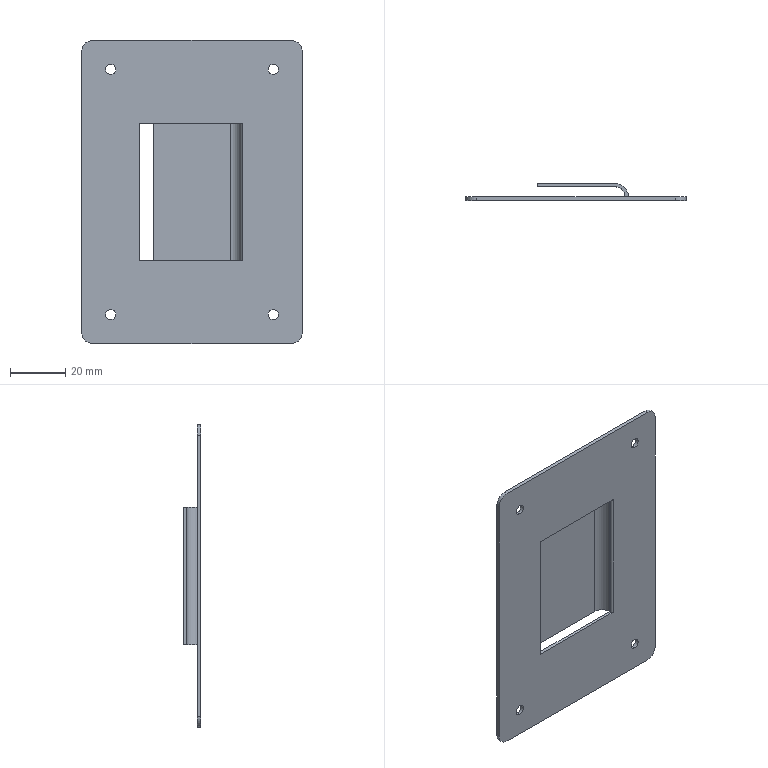Part | SolidWorks | features FlatPattern 1, ICE 1, SMBaseFlange 1, SheetMetal 1 | 1 solid | 30 faces | box 80 x 6.2 x 110 mm | volume 10376 mm3 | cylinder 15 | plane 15 | commonest cylinder face diameters 3.664 x8 8 x4 1.2 x1 7.6 x1 10 x1
STEP:
#1=CARTESIAN_POINT('',(-29.5,-1.2,-46.332));
#2=VERTEX_POINT('',#1);
#3=CARTESIAN_POINT('',(-29.5,-1.2,-42.668));
#4=VERTEX_POINT('',#3);
#5=CARTESIAN_POINT('',(-29.5,-1.2,-44.5));
#6=DIRECTION('',(0.,1.,0.));
#7=DIRECTION('',(0.,0.,-1.));
#8=AXIS2_PLACEMENT_3D('',#5,#6,#7);
#9=CIRCLE('',#8,1.832);
#10=EDGE_CURVE('',#2,#4,#9,.T.);
#11=ORIENTED_EDGE('',*,*,#10,.F.);
#12=CARTESIAN_POINT('',(-29.5,0.,-46.332));
#13=VERTEX_POINT('',#12);
#14=CARTESIAN_POINT('',(-29.5,-1.2,-46.332));
#15=DIRECTION('',(0.,1.,0.));
#16=VECTOR('',#15,1000.);
#17=LINE('',#14,#16);
#18=EDGE_CURVE('',#2,#13,#17,.T.);
#19=ORIENTED_EDGE('',*,*,#18,.T.);
#20=CARTESIAN_POINT('',(-29.5,0.,-42.668));
#21=VERTEX_POINT('',#20);
#22=CARTESIAN_POINT('',(-29.5,0.,-44.5));
#23=DIRECTION('',(0.,1.,0.));
#24=DIRECTION('',(0.,0.,-1.));
#25=AXIS2_PLACEMENT_3D('',#22,#23,#24);
#26=CIRCLE('',#25,1.832);
#27=EDGE_CURVE('',#13,#21,#26,.T.);
#28=ORIENTED_EDGE('',*,*,#27,.T.);
#29=CARTESIAN_POINT('',(-29.5,-1.2,-42.668));
#30=DIRECTION('',(0.,1.,0.));
#31=VECTOR('',#30,1000.);
#32=LINE('',#29,#31);
#33=EDGE_CURVE('',#4,#21,#32,.T.);
#34=ORIENTED_EDGE('',*,*,#33,.F.);
#35=EDGE_LOOP('',(#11,#19,#28,#34));
#36=FACE_OUTER_BOUND('',#35,.T.);
#37=CARTESIAN_POINT('',(-29.5,-1.2,-44.5));
#38=DIRECTION('',(0.,1.,0.));
#39=DIRECTION('',(0.,0.,1.));
#40=AXIS2_PLACEMENT_3D('',#37,#38,#39);
#41=CYLINDRICAL_SURFACE('',#40,1.832);
#42=ADVANCED_FACE('',(#36),#41,.F.);
#43=CARTESIAN_POINT('',(29.5,-1.2,-46.332));
#44=VERTEX_POINT('',#43);
#45=CARTESIAN_POINT('',(29.5,-1.2,-42.668));
#46=VERTEX_POINT('',#45);
#47=CARTESIAN_POINT('',(29.5,-1.2,-44.5));
#48=DIRECTION('',(0.,1.,0.));
#49=DIRECTION('',(0.,0.,1.));
#50=AXIS2_PLACEMENT_3D('',#47,#48,#49);
#51=CIRCLE('',#50,1.832);
#52=EDGE_CURVE('',#44,#46,#51,.T.);
#53=ORIENTED_EDGE('',*,*,#52,.F.);
#54=CARTESIAN_POINT('',(29.5,0.,-46.332));
#55=VERTEX_POINT('',#54);
#56=CARTESIAN_POINT('',(29.5,-1.2,-46.332));
#57=DIRECTION('',(0.,1.,0.));
#58=VECTOR('',#57,1000.);
#59=LINE('',#56,#58);
#60=EDGE_CURVE('',#44,#55,#59,.T.);
#61=ORIENTED_EDGE('',*,*,#60,.T.);
#62=CARTESIAN_POINT('',(29.5,0.,-42.668));
#63=VERTEX_POINT('',#62);
#64=CARTESIAN_POINT('',(29.5,0.,-44.5));
#65=DIRECTION('',(0.,1.,0.));
#66=DIRECTION('',(0.,0.,1.));
#67=AXIS2_PLACEMENT_3D('',#64,#65,#66);
#68=CIRCLE('',#67,1.832);
#69=EDGE_CURVE('',#55,#63,#68,.T.);
#70=ORIENTED_EDGE('',*,*,#69,.T.);
#71=CARTESIAN_POINT('',(29.5,-1.2,-42.668));
#72=DIRECTION('',(0.,1.,0.));
#73=VECTOR('',#72,1000.);
#74=LINE('',#71,#73);
#75=EDGE_CURVE('',#46,#63,#74,.T.);
#76=ORIENTED_EDGE('',*,*,#75,.F.);
#77=EDGE_LOOP('',(#53,#61,#70,#76));
#78=FACE_OUTER_BOUND('',#77,.T.);
#79=CARTESIAN_POINT('',(29.5,-1.2,-44.5));
#80=DIRECTION('',(0.,1.,0.));
#81=DIRECTION('',(0.,0.,1.));
#82=AXIS2_PLACEMENT_3D('',#79,#80,#81);
#83=CYLINDRICAL_SURFACE('',#82,1.832);
#84=ADVANCED_FACE('',(#78),#83,.F.);
#85=CARTESIAN_POINT('',(29.5,-1.2,42.668));
#86=VERTEX_POINT('',#85);
#87=CARTESIAN_POINT('',(29.5,-1.2,46.332));
#88=VERTEX_POINT('',#87);
#89=CARTESIAN_POINT('',(29.5,-1.2,44.5));
#90=DIRECTION('',(0.,1.,0.));
#91=DIRECTION('',(0.,0.,-1.));
#92=AXIS2_PLACEMENT_3D('',#89,#90,#91);
#93=CIRCLE('',#92,1.832);
#94=EDGE_CURVE('',#86,#88,#93,.T.);
#95=ORIENTED_EDGE('',*,*,#94,.F.);
#96=CARTESIAN_POINT('',(29.5,0.,42.668));
#97=VERTEX_POINT('',#96);
#98=CARTESIAN_POINT('',(29.5,-1.2,42.668));
#99=DIRECTION('',(0.,1.,0.));
#100=VECTOR('',#99,1000.);
#101=LINE('',#98,#100);
#102=EDGE_CURVE('',#86,#97,#101,.T.);
#103=ORIENTED_EDGE('',*,*,#102,.T.);
#104=CARTESIAN_POINT('',(29.5,0.,46.332));
#105=VERTEX_POINT('',#104);
#106=CARTESIAN_POINT('',(29.5,0.,44.5));
#107=DIRECTION('',(0.,1.,0.));
#108=DIRECTION('',(0.,0.,-1.));
#109=AXIS2_PLACEMENT_3D('',#106,#107,#108);
#110=CIRCLE('',#109,1.832);
#111=EDGE_CURVE('',#97,#105,#110,.T.);
#112=ORIENTED_EDGE('',*,*,#111,.T.);
#113=CARTESIAN_POINT('',(29.5,-1.2,46.332));
#114=DIRECTION('',(0.,1.,0.));
#115=VECTOR('',#114,1000.);
#116=LINE('',#113,#115);
#117=EDGE_CURVE('',#88,#105,#116,.T.);
#118=ORIENTED_EDGE('',*,*,#117,.F.);
#119=EDGE_LOOP('',(#95,#103,#112,#118));
#120=FACE_OUTER_BOUND('',#119,.T.);
#121=CARTESIAN_POINT('',(29.5,-1.2,44.5));
#122=DIRECTION('',(0.,1.,0.));
#123=DIRECTION('',(0.,0.,1.));
#124=AXIS2_PLACEMENT_3D('',#121,#122,#123);
#125=CYLINDRICAL_SURFACE('',#124,1.832);
#126=ADVANCED_FACE('',(#120),#125,.F.);
#127=CARTESIAN_POINT('',(-29.5,-1.2,42.668));
#128=VERTEX_POINT('',#127);
#129=CARTESIAN_POINT('',(-29.5,-1.2,46.332));
#130=VERTEX_POINT('',#129);
#131=CARTESIAN_POINT('',(-29.5,-1.2,44.5));
#132=DIRECTION('',(0.,1.,0.));
#133=DIRECTION('',(0.,0.,1.));
#134=AXIS2_PLACEMENT_3D('',#131,#132,#133);
#135=CIRCLE('',#134,1.832);
#136=EDGE_CURVE('',#128,#130,#135,.T.);
#137=ORIENTED_EDGE('',*,*,#136,.F.);
#138=CARTESIAN_POINT('',(-29.5,0.,42.668));
#139=VERTEX_POINT('',#138);
#140=CARTESIAN_POINT('',(-29.5,-1.2,42.668));
#141=DIRECTION('',(0.,1.,0.));
#142=VECTOR('',#141,1000.);
#143=LINE('',#140,#142);
#144=EDGE_CURVE('',#128,#139,#143,.T.);
#145=ORIENTED_EDGE('',*,*,#144,.T.);
#146=CARTESIAN_POINT('',(-29.5,0.,46.332));
#147=VERTEX_POINT('',#146);
#148=CARTESIAN_POINT('',(-29.5,0.,44.5));
#149=DIRECTION('',(0.,1.,0.));
#150=DIRECTION('',(0.,0.,1.));
#151=AXIS2_PLACEMENT_3D('',#148,#149,#150);
#152=CIRCLE('',#151,1.832);
#153=EDGE_CURVE('',#139,#147,#152,.T.);
#154=ORIENTED_EDGE('',*,*,#153,.T.);
#155=CARTESIAN_POINT('',(-29.5,-1.2,46.332));
#156=DIRECTION('',(0.,1.,0.));
#157=VECTOR('',#156,1000.);
#158=LINE('',#155,#157);
#159=EDGE_CURVE('',#130,#147,#158,.T.);
#160=ORIENTED_EDGE('',*,*,#159,.F.);
#161=EDGE_LOOP('',(#137,#145,#154,#160));
#162=FACE_OUTER_BOUND('',#161,.T.);
#163=CARTESIAN_POINT('',(-29.5,-1.2,44.5));
#164=DIRECTION('',(0.,1.,0.));
#165=DIRECTION('',(0.,0.,1.));
#166=AXIS2_PLACEMENT_3D('',#163,#164,#165);
#167=CYLINDRICAL_SURFACE('',#166,1.832);
#168=ADVANCED_FACE('',(#162),#167,.F.);
#169=CARTESIAN_POINT('',(17.8,0.,25.));
#170=VERTEX_POINT('',#169);
#171=CARTESIAN_POINT('',(17.8,-0.6,25.));
#172=VERTEX_POINT('',#171);
#173=CARTESIAN_POINT('',(17.8,-0.6,25.));
#174=DIRECTION('',(0.,-1.,0.));
#175=VECTOR('',#174,1000.);
#176=LINE('',#173,#175);
#177=EDGE_CURVE('',#170,#172,#176,.T.);
#178=ORIENTED_EDGE('',*,*,#177,.T.);
#179=CARTESIAN_POINT('',(18.4,-1.2,25.));
#180=VERTEX_POINT('',#179);
#181=CARTESIAN_POINT('',(18.4,-0.6,25.));
#182=DIRECTION('',(0.,0.,1.));
#183=DIRECTION('',(1.,0.,0.));
#184=AXIS2_PLACEMENT_3D('',#181,#182,#183);
#185=CIRCLE('',#184,0.6);
#186=EDGE_CURVE('',#172,#180,#185,.T.);
#187=ORIENTED_EDGE('',*,*,#186,.T.);
#188=CARTESIAN_POINT('',(-19.,-1.2,25.));
#189=VERTEX_POINT('',#188);
#190=CARTESIAN_POINT('',(-19.,-1.2,25.));
#191=DIRECTION('',(1.,0.,0.));
#192=VECTOR('',#191,1000.);
#193=LINE('',#190,#192);
#194=EDGE_CURVE('',#189,#180,#193,.T.);
#195=ORIENTED_EDGE('',*,*,#194,.F.);
#196=CARTESIAN_POINT('',(-19.,0.,25.));
#197=VERTEX_POINT('',#196);
#198=CARTESIAN_POINT('',(-19.,-1.2,25.));
#199=DIRECTION('',(0.,1.,0.));
#200=VECTOR('',#199,1000.);
#201=LINE('',#198,#200);
#202=EDGE_CURVE('',#189,#197,#201,.T.);
#203=ORIENTED_EDGE('',*,*,#202,.T.);
#204=CARTESIAN_POINT('',(-19.,0.,25.));
#205=DIRECTION('',(1.,0.,0.));
#206=VECTOR('',#205,1000.);
#207=LINE('',#204,#206);
#208=EDGE_CURVE('',#197,#170,#207,.T.);
#209=ORIENTED_EDGE('',*,*,#208,.T.);
#210=EDGE_LOOP('',(#178,#187,#195,#203,#209));
#211=FACE_OUTER_BOUND('',#210,.T.);
#212=CARTESIAN_POINT('',(-19.,-1.2,25.));
#213=DIRECTION('',(0.,0.,1.));
#214=DIRECTION('',(1.,0.,0.));
#215=AXIS2_PLACEMENT_3D('',#212,#213,#214);
#216=PLANE('',#215);
#217=ADVANCED_FACE('',(#211),#216,.F.);
#218=CARTESIAN_POINT('',(17.8,0.,-25.));
#219=VERTEX_POINT('',#218);
#220=CARTESIAN_POINT('',(17.8,-0.6,-25.));
#221=VERTEX_POINT('',#220);
#222=CARTESIAN_POINT('',(17.8,-0.6,-25.));
#223=DIRECTION('',(0.,-1.,0.));
#224=VECTOR('',#223,1000.);
#225=LINE('',#222,#224);
#226=EDGE_CURVE('',#219,#221,#225,.T.);
#227=ORIENTED_EDGE('',*,*,#226,.F.);
#228=CARTESIAN_POINT('',(-19.,0.,-25.));
#229=VERTEX_POINT('',#228);
#230=CARTESIAN_POINT('',(-19.,0.,-25.));
#231=DIRECTION('',(-1.,0.,0.));
#232=VECTOR('',#231,1000.);
#233=LINE('',#230,#232);
#234=EDGE_CURVE('',#219,#229,#233,.T.);
#235=ORIENTED_EDGE('',*,*,#234,.T.);
#236=CARTESIAN_POINT('',(-19.,-1.2,-25.));
#237=VERTEX_POINT('',#236);
#238=CARTESIAN_POINT('',(-19.,-1.2,-25.));
#239=DIRECTION('',(0.,1.,0.));
#240=VECTOR('',#239,1000.);
#241=LINE('',#238,#240);
#242=EDGE_CURVE('',#237,#229,#241,.T.);
#243=ORIENTED_EDGE('',*,*,#242,.F.);
#244=CARTESIAN_POINT('',(18.4,-1.2,-25.));
#245=VERTEX_POINT('',#244);
#246=CARTESIAN_POINT('',(-19.,-1.2,-25.));
#247=DIRECTION('',(-1.,0.,0.));
#248=VECTOR('',#247,1000.);
#249=LINE('',#246,#248);
#250=EDGE_CURVE('',#245,#237,#249,.T.);
#251=ORIENTED_EDGE('',*,*,#250,.F.);
#252=CARTESIAN_POINT('',(18.4,-0.6,-25.));
#253=DIRECTION('',(0.,0.,1.));
#254=DIRECTION('',(-1.,0.,0.));
#255=AXIS2_PLACEMENT_3D('',#252,#253,#254);
#256=CIRCLE('',#255,0.6);
#257=EDGE_CURVE('',#221,#245,#256,.T.);
#258=ORIENTED_EDGE('',*,*,#257,.F.);
#259=EDGE_LOOP('',(#227,#235,#243,#251,#258));
#260=FACE_OUTER_BOUND('',#259,.T.);
#261=CARTESIAN_POINT('',(-19.,-1.2,-25.));
#262=DIRECTION('',(0.,0.,-1.));
#263=DIRECTION('',(-1.,0.,0.));
#264=AXIS2_PLACEMENT_3D('',#261,#262,#263);
#265=PLANE('',#264);
#266=ADVANCED_FACE('',(#260),#265,.F.);
#267=CARTESIAN_POINT('',(-40.,0.,51.));
#268=VERTEX_POINT('',#267);
#269=CARTESIAN_POINT('',(-36.,0.,55.));
#270=VERTEX_POINT('',#269);
#271=CARTESIAN_POINT('',(-36.,0.,51.));
#272=DIRECTION('',(0.,1.,0.));
#273=DIRECTION('',(0.,0.,-1.));
#274=AXIS2_PLACEMENT_3D('',#271,#272,#273);
#275=CIRCLE('',#274,4.);
#276=EDGE_CURVE('',#268,#270,#275,.T.);
#277=ORIENTED_EDGE('',*,*,#276,.F.);
#278=CARTESIAN_POINT('',(-40.,-1.2,51.));
#279=VERTEX_POINT('',#278);
#280=CARTESIAN_POINT('',(-40.,-1.2,51.));
#281=DIRECTION('',(0.,1.,0.));
#282=VECTOR('',#281,1000.);
#283=LINE('',#280,#282);
#284=EDGE_CURVE('',#279,#268,#283,.T.);
#285=ORIENTED_EDGE('',*,*,#284,.F.);
#286=CARTESIAN_POINT('',(-36.,-1.2,55.));
#287=VERTEX_POINT('',#286);
#288=CARTESIAN_POINT('',(-36.,-1.2,51.));
#289=DIRECTION('',(0.,1.,0.));
#290=DIRECTION('',(0.,0.,-1.));
#291=AXIS2_PLACEMENT_3D('',#288,#289,#290);
#292=CIRCLE('',#291,4.);
#293=EDGE_CURVE('',#279,#287,#292,.T.);
#294=ORIENTED_EDGE('',*,*,#293,.T.);
#295=CARTESIAN_POINT('',(-36.,-1.2,55.));
#296=DIRECTION('',(0.,1.,0.));
#297=VECTOR('',#296,1000.);
#298=LINE('',#295,#297);
#299=EDGE_CURVE('',#287,#270,#298,.T.);
#300=ORIENTED_EDGE('',*,*,#299,.T.);
#301=EDGE_LOOP('',(#277,#285,#294,#300));
#302=FACE_OUTER_BOUND('',#301,.T.);
#303=CARTESIAN_POINT('',(-36.,-1.2,51.));
#304=DIRECTION('',(0.,1.,0.));
#305=DIRECTION('',(0.,0.,1.));
#306=AXIS2_PLACEMENT_3D('',#303,#304,#305);
#307=CYLINDRICAL_SURFACE('',#306,4.);
#308=ADVANCED_FACE('',(#302),#307,.T.);
#309=CARTESIAN_POINT('',(-40.,0.,-51.));
#310=VERTEX_POINT('',#309);
#311=CARTESIAN_POINT('',(-40.,0.,51.));
#312=DIRECTION('',(0.,0.,1.));
#313=VECTOR('',#312,1000.);
#314=LINE('',#311,#313);
#315=EDGE_CURVE('',#310,#268,#314,.T.);
#316=ORIENTED_EDGE('',*,*,#315,.F.);
#317=CARTESIAN_POINT('',(-40.,-1.2,-51.));
#318=VERTEX_POINT('',#317);
#319=CARTESIAN_POINT('',(-40.,-1.2,-51.));
#320=DIRECTION('',(0.,1.,0.));
#321=VECTOR('',#320,1000.);
#322=LINE('',#319,#321);
#323=EDGE_CURVE('',#318,#310,#322,.T.);
#324=ORIENTED_EDGE('',*,*,#323,.F.);
#325=CARTESIAN_POINT('',(-40.,-1.2,51.));
#326=DIRECTION('',(0.,0.,1.));
#327=VECTOR('',#326,1000.);
#328=LINE('',#325,#327);
#329=EDGE_CURVE('',#318,#279,#328,.T.);
#330=ORIENTED_EDGE('',*,*,#329,.T.);
#331=ORIENTED_EDGE('',*,*,#284,.T.);
#332=EDGE_LOOP('',(#316,#324,#330,#331));
#333=FACE_OUTER_BOUND('',#332,.T.);
#334=CARTESIAN_POINT('',(-40.,-1.2,51.));
#335=DIRECTION('',(-1.,0.,0.));
#336=DIRECTION('',(0.,0.,1.));
#337=AXIS2_PLACEMENT_3D('',#334,#335,#336);
#338=PLANE('',#337);
#339=ADVANCED_FACE('',(#333),#338,.T.);
#340=CARTESIAN_POINT('',(-36.,0.,-55.));
#341=VERTEX_POINT('',#340);
#342=CARTESIAN_POINT('',(-36.,0.,-51.));
#343=DIRECTION('',(0.,1.,0.));
#344=DIRECTION('',(0.,0.,-1.));
#345=AXIS2_PLACEMENT_3D('',#342,#343,#344);
#346=CIRCLE('',#345,4.);
#347=EDGE_CURVE('',#341,#310,#346,.T.);
#348=ORIENTED_EDGE('',*,*,#347,.F.);
#349=CARTESIAN_POINT('',(-36.,-1.2,-55.));
#350=VERTEX_POINT('',#349);
#351=CARTESIAN_POINT('',(-36.,-1.2,-55.));
#352=DIRECTION('',(0.,1.,0.));
#353=VECTOR('',#352,1000.);
#354=LINE('',#351,#353);
#355=EDGE_CURVE('',#350,#341,#354,.T.);
#356=ORIENTED_EDGE('',*,*,#355,.F.);
#357=CARTESIAN_POINT('',(-36.,-1.2,-51.));
#358=DIRECTION('',(0.,1.,0.));
#359=DIRECTION('',(0.,0.,-1.));
#360=AXIS2_PLACEMENT_3D('',#357,#358,#359);
#361=CIRCLE('',#360,4.);
#362=EDGE_CURVE('',#350,#318,#361,.T.);
#363=ORIENTED_EDGE('',*,*,#362,.T.);
#364=ORIENTED_EDGE('',*,*,#323,.T.);
#365=EDGE_LOOP('',(#348,#356,#363,#364));
#366=FACE_OUTER_BOUND('',#365,.T.);
#367=CARTESIAN_POINT('',(-36.,-1.2,-51.));
#368=DIRECTION('',(0.,1.,0.));
#369=DIRECTION('',(0.,0.,1.));
#370=AXIS2_PLACEMENT_3D('',#367,#368,#369);
#371=CYLINDRICAL_SURFACE('',#370,4.);
#372=ADVANCED_FACE('',(#366),#371,.T.);
#373=CARTESIAN_POINT('',(36.,0.,-55.));
#374=VERTEX_POINT('',#373);
#375=CARTESIAN_POINT('',(-36.,0.,-55.));
#376=DIRECTION('',(-1.,0.,0.));
#377=VECTOR('',#376,1000.);
#378=LINE('',#375,#377);
#379=EDGE_CURVE('',#374,#341,#378,.T.);
#380=ORIENTED_EDGE('',*,*,#379,.F.);
#381=CARTESIAN_POINT('',(36.,-1.2,-55.));
#382=VERTEX_POINT('',#381);
#383=CARTESIAN_POINT('',(36.,-1.2,-55.));
#384=DIRECTION('',(0.,1.,0.));
#385=VECTOR('',#384,1000.);
#386=LINE('',#383,#385);
#387=EDGE_CURVE('',#382,#374,#386,.T.);
#388=ORIENTED_EDGE('',*,*,#387,.F.);
#389=CARTESIAN_POINT('',(-36.,-1.2,-55.));
#390=DIRECTION('',(-1.,0.,0.));
#391=VECTOR('',#390,1000.);
#392=LINE('',#389,#391);
#393=EDGE_CURVE('',#382,#350,#392,.T.);
#394=ORIENTED_EDGE('',*,*,#393,.T.);
#395=ORIENTED_EDGE('',*,*,#355,.T.);
#396=EDGE_LOOP('',(#380,#388,#394,#395));
#397=FACE_OUTER_BOUND('',#396,.T.);
#398=CARTESIAN_POINT('',(-36.,-1.2,-55.));
#399=DIRECTION('',(0.,0.,-1.));
#400=DIRECTION('',(-1.,0.,0.));
#401=AXIS2_PLACEMENT_3D('',#398,#399,#400);
#402=PLANE('',#401);
#403=ADVANCED_FACE('',(#397),#402,.T.);
#404=CARTESIAN_POINT('',(40.,0.,-51.));
#405=VERTEX_POINT('',#404);
#406=CARTESIAN_POINT('',(36.,0.,-51.));
#407=DIRECTION('',(0.,1.,0.));
#408=DIRECTION('',(0.,0.,1.));
#409=AXIS2_PLACEMENT_3D('',#406,#407,#408);
#410=CIRCLE('',#409,4.);
#411=EDGE_CURVE('',#405,#374,#410,.T.);
#412=ORIENTED_EDGE('',*,*,#411,.F.);
#413=CARTESIAN_POINT('',(40.,-1.2,-51.));
#414=VERTEX_POINT('',#413);
#415=CARTESIAN_POINT('',(40.,-1.2,-51.));
#416=DIRECTION('',(0.,1.,0.));
#417=VECTOR('',#416,1000.);
#418=LINE('',#415,#417);
#419=EDGE_CURVE('',#414,#405,#418,.T.);
#420=ORIENTED_EDGE('',*,*,#419,.F.);
#421=CARTESIAN_POINT('',(36.,-1.2,-51.));
#422=DIRECTION('',(0.,1.,0.));
#423=DIRECTION('',(0.,0.,1.));
#424=AXIS2_PLACEMENT_3D('',#421,#422,#423);
#425=CIRCLE('',#424,4.);
#426=EDGE_CURVE('',#414,#382,#425,.T.);
#427=ORIENTED_EDGE('',*,*,#426,.T.);
#428=ORIENTED_EDGE('',*,*,#387,.T.);
#429=EDGE_LOOP('',(#412,#420,#427,#428));
#430=FACE_OUTER_BOUND('',#429,.T.);
#431=CARTESIAN_POINT('',(36.,-1.2,-51.));
#432=DIRECTION('',(0.,1.,0.));
#433=DIRECTION('',(0.,0.,1.));
#434=AXIS2_PLACEMENT_3D('',#431,#432,#433);
#435=CYLINDRICAL_SURFACE('',#434,4.);
#436=ADVANCED_FACE('',(#430),#435,.T.);
#437=CARTESIAN_POINT('',(40.,0.,51.));
#438=VERTEX_POINT('',#437);
#439=CARTESIAN_POINT('',(40.,0.,51.));
#440=DIRECTION('',(0.,0.,-1.));
#441=VECTOR('',#440,1000.);
#442=LINE('',#439,#441);
#443=EDGE_CURVE('',#438,#405,#442,.T.);
#444=ORIENTED_EDGE('',*,*,#443,.F.);
#445=CARTESIAN_POINT('',(40.,-1.2,51.));
#446=VERTEX_POINT('',#445);
#447=CARTESIAN_POINT('',(40.,-1.2,51.));
#448=DIRECTION('',(0.,1.,0.));
#449=VECTOR('',#448,1000.);
#450=LINE('',#447,#449);
#451=EDGE_CURVE('',#446,#438,#450,.T.);
#452=ORIENTED_EDGE('',*,*,#451,.F.);
#453=CARTESIAN_POINT('',(40.,-1.2,51.));
#454=DIRECTION('',(0.,0.,-1.));
#455=VECTOR('',#454,1000.);
#456=LINE('',#453,#455);
#457=EDGE_CURVE('',#446,#414,#456,.T.);
#458=ORIENTED_EDGE('',*,*,#457,.T.);
#459=ORIENTED_EDGE('',*,*,#419,.T.);
#460=EDGE_LOOP('',(#444,#452,#458,#459));
#461=FACE_OUTER_BOUND('',#460,.T.);
#462=CARTESIAN_POINT('',(40.,-1.2,51.));
#463=DIRECTION('',(1.,0.,0.));
#464=DIRECTION('',(0.,0.,-1.));
#465=AXIS2_PLACEMENT_3D('',#462,#463,#464);
#466=PLANE('',#465);
#467=ADVANCED_FACE('',(#461),#466,.T.);
#468=CARTESIAN_POINT('',(36.,0.,55.));
#469=VERTEX_POINT('',#468);
#470=CARTESIAN_POINT('',(36.,0.,51.));
#471=DIRECTION('',(0.,1.,0.));
#472=DIRECTION('',(0.,0.,1.));
#473=AXIS2_PLACEMENT_3D('',#470,#471,#472);
#474=CIRCLE('',#473,4.);
#475=EDGE_CURVE('',#469,#438,#474,.T.);
#476=ORIENTED_EDGE('',*,*,#475,.F.);
#477=CARTESIAN_POINT('',(36.,-1.2,55.));
#478=VERTEX_POINT('',#477);
#479=CARTESIAN_POINT('',(36.,-1.2,55.));
#480=DIRECTION('',(0.,1.,0.));
#481=VECTOR('',#480,1000.);
#482=LINE('',#479,#481);
#483=EDGE_CURVE('',#478,#469,#482,.T.);
#484=ORIENTED_EDGE('',*,*,#483,.F.);
#485=CARTESIAN_POINT('',(36.,-1.2,51.));
#486=DIRECTION('',(0.,1.,0.));
#487=DIRECTION('',(0.,0.,1.));
#488=AXIS2_PLACEMENT_3D('',#485,#486,#487);
#489=CIRCLE('',#488,4.);
#490=EDGE_CURVE('',#478,#446,#489,.T.);
#491=ORIENTED_EDGE('',*,*,#490,.T.);
#492=ORIENTED_EDGE('',*,*,#451,.T.);
#493=EDGE_LOOP('',(#476,#484,#491,#492));
#494=FACE_OUTER_BOUND('',#493,.T.);
#495=CARTESIAN_POINT('',(36.,-1.2,51.));
#496=DIRECTION('',(0.,1.,0.));
#497=DIRECTION('',(0.,0.,1.));
#498=AXIS2_PLACEMENT_3D('',#495,#496,#497);
#499=CYLINDRICAL_SURFACE('',#498,4.);
#500=ADVANCED_FACE('',(#494),#499,.T.);
#501=CARTESIAN_POINT('',(-36.,0.,55.));
#502=DIRECTION('',(1.,0.,0.));
#503=VECTOR('',#502,1000.);
#504=LINE('',#501,#503);
#505=EDGE_CURVE('',#270,#469,#504,.T.);
#506=ORIENTED_EDGE('',*,*,#505,.F.);
#507=ORIENTED_EDGE('',*,*,#299,.F.);
#508=CARTESIAN_POINT('',(-36.,-1.2,55.));
#509=DIRECTION('',(1.,0.,0.));
#510=VECTOR('',#509,1000.);
#511=LINE('',#508,#510);
#512=EDGE_CURVE('',#287,#478,#511,.T.);
#513=ORIENTED_EDGE('',*,*,#512,.T.);
#514=ORIENTED_EDGE('',*,*,#483,.T.);
#515=EDGE_LOOP('',(#506,#507,#513,#514));
#516=FACE_OUTER_BOUND('',#515,.T.);
#517=CARTESIAN_POINT('',(-36.,-1.2,55.));
#518=DIRECTION('',(0.,0.,1.));
#519=DIRECTION('',(1.,0.,0.));
#520=AXIS2_PLACEMENT_3D('',#517,#518,#519);
#521=PLANE('',#520);
#522=ADVANCED_FACE('',(#516),#521,.T.);
#523=CARTESIAN_POINT('',(18.4,-1.2,58.577));
#524=DIRECTION('',(0.,0.,-1.));
#525=VECTOR('',#524,1000.);
#526=LINE('',#523,#525);
#527=EDGE_CURVE('',#180,#245,#526,.T.);
#528=ORIENTED_EDGE('',*,*,#527,.T.);
#529=ORIENTED_EDGE('',*,*,#250,.T.);
#530=CARTESIAN_POINT('',(-19.,-1.2,-25.));
#531=DIRECTION('',(0.,0.,1.));
#532=VECTOR('',#531,1000.);
#533=LINE('',#530,#532);
#534=EDGE_CURVE('',#237,#189,#533,.T.);
#535=ORIENTED_EDGE('',*,*,#534,.T.);
#536=ORIENTED_EDGE('',*,*,#194,.T.);
#537=EDGE_LOOP('',(#528,#529,#535,#536));
#538=FACE_BOUND('',#537,.T.);
#539=CARTESIAN_POINT('',(-29.5,-1.2,-44.5));
#540=DIRECTION('',(0.,1.,0.));
#541=DIRECTION('',(0.,0.,-1.));
#542=AXIS2_PLACEMENT_3D('',#539,#540,#541);
#543=CIRCLE('',#542,1.832);
#544=EDGE_CURVE('',#4,#2,#543,.T.);
#545=ORIENTED_EDGE('',*,*,#544,.T.);
#546=ORIENTED_EDGE('',*,*,#10,.T.);
#547=EDGE_LOOP('',(#545,#546));
#548=FACE_BOUND('',#547,.T.);
#549=CARTESIAN_POINT('',(29.5,-1.2,-44.5));
#550=DIRECTION('',(0.,1.,0.));
#551=DIRECTION('',(0.,0.,1.));
#552=AXIS2_PLACEMENT_3D('',#549,#550,#551);
#553=CIRCLE('',#552,1.832);
#554=EDGE_CURVE('',#46,#44,#553,.T.);
#555=ORIENTED_EDGE('',*,*,#554,.T.);
#556=ORIENTED_EDGE('',*,*,#52,.T.);
#557=EDGE_LOOP('',(#555,#556));
#558=FACE_BOUND('',#557,.T.);
#559=CARTESIAN_POINT('',(29.5,-1.2,44.5));
#560=DIRECTION('',(0.,1.,0.));
#561=DIRECTION('',(0.,0.,-1.));
#562=AXIS2_PLACEMENT_3D('',#559,#560,#561);
#563=CIRCLE('',#562,1.832);
#564=EDGE_CURVE('',#88,#86,#563,.T.);
#565=ORIENTED_EDGE('',*,*,#564,.T.);
#566=ORIENTED_EDGE('',*,*,#94,.T.);
#567=EDGE_LOOP('',(#565,#566));
#568=FACE_BOUND('',#567,.T.);
#569=CARTESIAN_POINT('',(-29.5,-1.2,44.5));
#570=DIRECTION('',(0.,1.,0.));
#571=DIRECTION('',(0.,0.,1.));
#572=AXIS2_PLACEMENT_3D('',#569,#570,#571);
#573=CIRCLE('',#572,1.832);
#574=EDGE_CURVE('',#130,#128,#573,.T.);
#575=ORIENTED_EDGE('',*,*,#574,.T.);
#576=ORIENTED_EDGE('',*,*,#136,.T.);
#577=EDGE_LOOP('',(#575,#576));
#578=FACE_BOUND('',#577,.T.);
#579=ORIENTED_EDGE('',*,*,#293,.F.);
#580=ORIENTED_EDGE('',*,*,#329,.F.);
#581=ORIENTED_EDGE('',*,*,#362,.F.);
#582=ORIENTED_EDGE('',*,*,#393,.F.);
#583=ORIENTED_EDGE('',*,*,#426,.F.);
#584=ORIENTED_EDGE('',*,*,#457,.F.);
#585=ORIENTED_EDGE('',*,*,#490,.F.);
#586=ORIENTED_EDGE('',*,*,#512,.F.);
#587=EDGE_LOOP('',(#579,#580,#581,#582,#583,#584,#585,#586));
#588=FACE_OUTER_BOUND('',#587,.T.);
#589=CARTESIAN_POINT('',(-36.,-1.2,51.));
#590=DIRECTION('',(0.,-1.,0.));
#591=DIRECTION('',(0.,0.,-1.));
#592=AXIS2_PLACEMENT_3D('',#589,#590,#591);
#593=PLANE('',#592);
#594=ADVANCED_FACE('',(#538,#548,#558,#568,#578,#588),#593,.T.);
#595=CARTESIAN_POINT('',(19.,0.,25.));
#596=VERTEX_POINT('',#595);
#597=CARTESIAN_POINT('',(19.,0.,-25.));
#598=VERTEX_POINT('',#597);
#599=CARTESIAN_POINT('',(19.,0.,-25.));
#600=DIRECTION('',(0.,0.,-1.));
#601=VECTOR('',#600,1000.);
#602=LINE('',#599,#601);
#603=EDGE_CURVE('',#596,#598,#602,.T.);
#604=ORIENTED_EDGE('',*,*,#603,.F.);
#605=CARTESIAN_POINT('',(-36.,0.,25.));
#606=DIRECTION('',(-1.,0.,0.));
#607=VECTOR('',#606,1000.);
#608=LINE('',#605,#607);
#609=EDGE_CURVE('',#596,#170,#608,.T.);
#610=ORIENTED_EDGE('',*,*,#609,.T.);
#611=ORIENTED_EDGE('',*,*,#208,.F.);
#612=CARTESIAN_POINT('',(-19.,0.,-25.));
#613=DIRECTION('',(0.,0.,1.));
#614=VECTOR('',#613,1000.);
#615=LINE('',#612,#614);
#616=EDGE_CURVE('',#229,#197,#615,.T.);
#617=ORIENTED_EDGE('',*,*,#616,.F.);
#618=ORIENTED_EDGE('',*,*,#234,.F.);
#619=CARTESIAN_POINT('',(-19.,0.,-25.));
#620=DIRECTION('',(-1.,0.,0.));
#621=VECTOR('',#620,1000.);
#622=LINE('',#619,#621);
#623=EDGE_CURVE('',#598,#219,#622,.T.);
#624=ORIENTED_EDGE('',*,*,#623,.F.);
#625=EDGE_LOOP('',(#604,#610,#611,#617,#618,#624));
#626=FACE_BOUND('',#625,.T.);
#627=CARTESIAN_POINT('',(-29.5,0.,-44.5));
#628=DIRECTION('',(0.,1.,0.));
#629=DIRECTION('',(0.,0.,-1.));
#630=AXIS2_PLACEMENT_3D('',#627,#628,#629);
#631=CIRCLE('',#630,1.832);
#632=EDGE_CURVE('',#21,#13,#631,.T.);
#633=ORIENTED_EDGE('',*,*,#632,.F.);
#634=ORIENTED_EDGE('',*,*,#27,.F.);
#635=EDGE_LOOP('',(#633,#634));
#636=FACE_BOUND('',#635,.T.);
#637=CARTESIAN_POINT('',(29.5,0.,-44.5));
#638=DIRECTION('',(0.,1.,0.));
#639=DIRECTION('',(0.,0.,1.));
#640=AXIS2_PLACEMENT_3D('',#637,#638,#639);
#641=CIRCLE('',#640,1.832);
#642=EDGE_CURVE('',#63,#55,#641,.T.);
#643=ORIENTED_EDGE('',*,*,#642,.F.);
#644=ORIENTED_EDGE('',*,*,#69,.F.);
#645=EDGE_LOOP('',(#643,#644));
#646=FACE_BOUND('',#645,.T.);
#647=CARTESIAN_POINT('',(29.5,0.,44.5));
#648=DIRECTION('',(0.,1.,0.));
#649=DIRECTION('',(0.,0.,-1.));
#650=AXIS2_PLACEMENT_3D('',#647,#648,#649);
#651=CIRCLE('',#650,1.832);
#652=EDGE_CURVE('',#105,#97,#651,.T.);
#653=ORIENTED_EDGE('',*,*,#652,.F.);
#654=ORIENTED_EDGE('',*,*,#111,.F.);
#655=EDGE_LOOP('',(#653,#654));
#656=FACE_BOUND('',#655,.T.);
#657=CARTESIAN_POINT('',(-29.5,0.,44.5));
#658=DIRECTION('',(0.,1.,0.));
#659=DIRECTION('',(0.,0.,1.));
#660=AXIS2_PLACEMENT_3D('',#657,#658,#659);
#661=CIRCLE('',#660,1.832);
#662=EDGE_CURVE('',#147,#139,#661,.T.);
#663=ORIENTED_EDGE('',*,*,#662,.F.);
#664=ORIENTED_EDGE('',*,*,#153,.F.);
#665=EDGE_LOOP('',(#663,#664));
#666=FACE_BOUND('',#665,.T.);
#667=ORIENTED_EDGE('',*,*,#276,.T.);
#668=ORIENTED_EDGE('',*,*,#505,.T.);
#669=ORIENTED_EDGE('',*,*,#475,.T.);
#670=ORIENTED_EDGE('',*,*,#443,.T.);
#671=ORIENTED_EDGE('',*,*,#411,.T.);
#672=ORIENTED_EDGE('',*,*,#379,.T.);
#673=ORIENTED_EDGE('',*,*,#347,.T.);
#674=ORIENTED_EDGE('',*,*,#315,.T.);
#675=EDGE_LOOP('',(#667,#668,#669,#670,#671,#672,#673,#674));
#676=FACE_OUTER_BOUND('',#675,.T.);
#677=CARTESIAN_POINT('',(-36.,0.,51.));
#678=DIRECTION('',(0.,-1.,0.));
#679=DIRECTION('',(0.,0.,-1.));
#680=AXIS2_PLACEMENT_3D('',#677,#678,#679);
#681=PLANE('',#680);
#682=ADVANCED_FACE('',(#626,#636,#646,#656,#666,#676),#681,.F.);
#683=ORIENTED_EDGE('',*,*,#144,.F.);
#684=ORIENTED_EDGE('',*,*,#574,.F.);
#685=ORIENTED_EDGE('',*,*,#159,.T.);
#686=ORIENTED_EDGE('',*,*,#662,.T.);
#687=EDGE_LOOP('',(#683,#684,#685,#686));
#688=FACE_OUTER_BOUND('',#687,.T.);
#689=CARTESIAN_POINT('',(-29.5,-1.2,44.5));
#690=DIRECTION('',(0.,1.,0.));
#691=DIRECTION('',(0.,0.,1.));
#692=AXIS2_PLACEMENT_3D('',#689,#690,#691);
#693=CYLINDRICAL_SURFACE('',#692,1.832);
#694=ADVANCED_FACE('',(#688),#693,.F.);
#695=ORIENTED_EDGE('',*,*,#102,.F.);
#696=ORIENTED_EDGE('',*,*,#564,.F.);
#697=ORIENTED_EDGE('',*,*,#117,.T.);
#698=ORIENTED_EDGE('',*,*,#652,.T.);
#699=EDGE_LOOP('',(#695,#696,#697,#698));
#700=FACE_OUTER_BOUND('',#699,.T.);
#701=CARTESIAN_POINT('',(29.5,-1.2,44.5));
#702=DIRECTION('',(0.,1.,0.));
#703=DIRECTION('',(0.,0.,1.));
#704=AXIS2_PLACEMENT_3D('',#701,#702,#703);
#705=CYLINDRICAL_SURFACE('',#704,1.832);
#706=ADVANCED_FACE('',(#700),#705,.F.);
#707=ORIENTED_EDGE('',*,*,#60,.F.);
#708=ORIENTED_EDGE('',*,*,#554,.F.);
#709=ORIENTED_EDGE('',*,*,#75,.T.);
#710=ORIENTED_EDGE('',*,*,#642,.T.);
#711=EDGE_LOOP('',(#707,#708,#709,#710));
#712=FACE_OUTER_BOUND('',#711,.T.);
#713=CARTESIAN_POINT('',(29.5,-1.2,-44.5));
#714=DIRECTION('',(0.,1.,0.));
#715=DIRECTION('',(0.,0.,1.));
#716=AXIS2_PLACEMENT_3D('',#713,#714,#715);
#717=CYLINDRICAL_SURFACE('',#716,1.832);
#718=ADVANCED_FACE('',(#712),#717,.F.);
#719=ORIENTED_EDGE('',*,*,#18,.F.);
#720=ORIENTED_EDGE('',*,*,#544,.F.);
#721=ORIENTED_EDGE('',*,*,#33,.T.);
#722=ORIENTED_EDGE('',*,*,#632,.T.);
#723=EDGE_LOOP('',(#719,#720,#721,#722));
#724=FACE_OUTER_BOUND('',#723,.T.);
#725=CARTESIAN_POINT('',(-29.5,-1.2,-44.5));
#726=DIRECTION('',(0.,1.,0.));
#727=DIRECTION('',(0.,0.,1.));
#728=AXIS2_PLACEMENT_3D('',#725,#726,#727);
#729=CYLINDRICAL_SURFACE('',#728,1.832);
#730=ADVANCED_FACE('',(#724),#729,.F.);
#731=ORIENTED_EDGE('',*,*,#616,.T.);
#732=ORIENTED_EDGE('',*,*,#202,.F.);
#733=ORIENTED_EDGE('',*,*,#534,.F.);
#734=ORIENTED_EDGE('',*,*,#242,.T.);
#735=EDGE_LOOP('',(#731,#732,#733,#734));
#736=FACE_OUTER_BOUND('',#735,.T.);
#737=CARTESIAN_POINT('',(-19.,-1.2,-25.));
#738=DIRECTION('',(-1.,0.,0.));
#739=DIRECTION('',(0.,0.,1.));
#740=AXIS2_PLACEMENT_3D('',#737,#738,#739);
#741=PLANE('',#740);
#742=ADVANCED_FACE('',(#736),#741,.F.);
#743=ORIENTED_EDGE('',*,*,#609,.F.);
#744=CARTESIAN_POINT('',(14.,5.,25.));
#745=VERTEX_POINT('',#744);
#746=CARTESIAN_POINT('',(14.,0.,25.));
#747=DIRECTION('',(0.,0.,1.));
#748=DIRECTION('',(1.,0.,0.));
#749=AXIS2_PLACEMENT_3D('',#746,#747,#748);
#750=CIRCLE('',#749,5.);
#751=EDGE_CURVE('',#596,#745,#750,.T.);
#752=ORIENTED_EDGE('',*,*,#751,.T.);
#753=CARTESIAN_POINT('',(-14.,5.,25.));
#754=VERTEX_POINT('',#753);
#755=CARTESIAN_POINT('',(14.,5.,25.));
#756=DIRECTION('',(-1.,0.,0.));
#757=VECTOR('',#756,1000.);
#758=LINE('',#755,#757);
#759=EDGE_CURVE('',#745,#754,#758,.T.);
#760=ORIENTED_EDGE('',*,*,#759,.T.);
#761=CARTESIAN_POINT('',(-14.,3.8,25.));
#762=VERTEX_POINT('',#761);
#763=CARTESIAN_POINT('',(-14.,5.,25.));
#764=DIRECTION('',(0.,-1.,0.));
#765=VECTOR('',#764,1000.);
#766=LINE('',#763,#765);
#767=EDGE_CURVE('',#754,#762,#766,.T.);
#768=ORIENTED_EDGE('',*,*,#767,.T.);
#769=CARTESIAN_POINT('',(14.,3.8,25.));
#770=VERTEX_POINT('',#769);
#771=CARTESIAN_POINT('',(14.,3.8,25.));
#772=DIRECTION('',(1.,0.,0.));
#773=VECTOR('',#772,1000.);
#774=LINE('',#771,#773);
#775=EDGE_CURVE('',#762,#770,#774,.T.);
#776=ORIENTED_EDGE('',*,*,#775,.T.);
#777=CARTESIAN_POINT('',(14.,0.,25.));
#778=DIRECTION('',(0.,0.,-1.));
#779=DIRECTION('',(1.,0.,0.));
#780=AXIS2_PLACEMENT_3D('',#777,#778,#779);
#781=CIRCLE('',#780,3.8);
#782=EDGE_CURVE('',#770,#170,#781,.T.);
#783=ORIENTED_EDGE('',*,*,#782,.T.);
#784=EDGE_LOOP('',(#743,#752,#760,#768,#776,#783));
#785=FACE_OUTER_BOUND('',#784,.T.);
#786=CARTESIAN_POINT('',(-19.,-1.2,25.));
#787=DIRECTION('',(0.,0.,1.));
#788=DIRECTION('',(1.,0.,0.));
#789=AXIS2_PLACEMENT_3D('',#786,#787,#788);
#790=PLANE('',#789);
#791=ADVANCED_FACE('',(#785),#790,.T.);
#792=ORIENTED_EDGE('',*,*,#623,.T.);
#793=CARTESIAN_POINT('',(14.,3.8,-25.));
#794=VERTEX_POINT('',#793);
#795=CARTESIAN_POINT('',(14.,0.,-25.));
#796=DIRECTION('',(0.,0.,-1.));
#797=DIRECTION('',(-1.,0.,0.));
#798=AXIS2_PLACEMENT_3D('',#795,#796,#797);
#799=CIRCLE('',#798,3.8);
#800=EDGE_CURVE('',#794,#219,#799,.T.);
#801=ORIENTED_EDGE('',*,*,#800,.F.);
#802=CARTESIAN_POINT('',(-14.,3.8,-25.));
#803=VERTEX_POINT('',#802);
#804=CARTESIAN_POINT('',(14.,3.8,-25.));
#805=DIRECTION('',(1.,0.,0.));
#806=VECTOR('',#805,1000.);
#807=LINE('',#804,#806);
#808=EDGE_CURVE('',#803,#794,#807,.T.);
#809=ORIENTED_EDGE('',*,*,#808,.F.);
#810=CARTESIAN_POINT('',(-14.,5.,-25.));
#811=VERTEX_POINT('',#810);
#812=CARTESIAN_POINT('',(-14.,5.,-25.));
#813=DIRECTION('',(0.,-1.,0.));
#814=VECTOR('',#813,1000.);
#815=LINE('',#812,#814);
#816=EDGE_CURVE('',#811,#803,#815,.T.);
#817=ORIENTED_EDGE('',*,*,#816,.F.);
#818=CARTESIAN_POINT('',(14.,5.,-25.));
#819=VERTEX_POINT('',#818);
#820=CARTESIAN_POINT('',(14.,5.,-25.));
#821=DIRECTION('',(-1.,0.,0.));
#822=VECTOR('',#821,1000.);
#823=LINE('',#820,#822);
#824=EDGE_CURVE('',#819,#811,#823,.T.);
#825=ORIENTED_EDGE('',*,*,#824,.F.);
#826=CARTESIAN_POINT('',(14.,0.,-25.));
#827=DIRECTION('',(0.,0.,1.));
#828=DIRECTION('',(-1.,0.,0.));
#829=AXIS2_PLACEMENT_3D('',#826,#827,#828);
#830=CIRCLE('',#829,5.);
#831=EDGE_CURVE('',#598,#819,#830,.T.);
#832=ORIENTED_EDGE('',*,*,#831,.F.);
#833=EDGE_LOOP('',(#792,#801,#809,#817,#825,#832));
#834=FACE_OUTER_BOUND('',#833,.T.);
#835=CARTESIAN_POINT('',(-19.,-1.2,-25.));
#836=DIRECTION('',(0.,0.,-1.));
#837=DIRECTION('',(-1.,0.,0.));
#838=AXIS2_PLACEMENT_3D('',#835,#836,#837);
#839=PLANE('',#838);
#840=ADVANCED_FACE('',(#834),#839,.T.);
#841=ORIENTED_EDGE('',*,*,#751,.F.);
#842=ORIENTED_EDGE('',*,*,#603,.T.);
#843=ORIENTED_EDGE('',*,*,#831,.T.);
#844=CARTESIAN_POINT('',(14.,5.,58.577));
#845=DIRECTION('',(0.,0.,-1.));
#846=VECTOR('',#845,1000.);
#847=LINE('',#844,#846);
#848=EDGE_CURVE('',#745,#819,#847,.T.);
#849=ORIENTED_EDGE('',*,*,#848,.F.);
#850=EDGE_LOOP('',(#841,#842,#843,#849));
#851=FACE_OUTER_BOUND('',#850,.T.);
#852=CARTESIAN_POINT('',(14.,0.,58.577));
#853=DIRECTION('',(0.,0.,-1.));
#854=DIRECTION('',(-1.,0.,0.));
#855=AXIS2_PLACEMENT_3D('',#852,#853,#854);
#856=CYLINDRICAL_SURFACE('',#855,5.);
#857=ADVANCED_FACE('',(#851),#856,.T.);
#858=ORIENTED_EDGE('',*,*,#759,.F.);
#859=ORIENTED_EDGE('',*,*,#848,.T.);
#860=ORIENTED_EDGE('',*,*,#824,.T.);
#861=CARTESIAN_POINT('',(-14.,5.,58.577));
#862=DIRECTION('',(0.,0.,-1.));
#863=VECTOR('',#862,1000.);
#864=LINE('',#861,#863);
#865=EDGE_CURVE('',#754,#811,#864,.T.);
#866=ORIENTED_EDGE('',*,*,#865,.F.);
#867=EDGE_LOOP('',(#858,#859,#860,#866));
#868=FACE_OUTER_BOUND('',#867,.T.);
#869=CARTESIAN_POINT('',(14.,5.,58.577));
#870=DIRECTION('',(0.,-1.,0.));
#871=DIRECTION('',(1.,0.,0.));
#872=AXIS2_PLACEMENT_3D('',#869,#870,#871);
#873=PLANE('',#872);
#874=ADVANCED_FACE('',(#868),#873,.F.);
#875=ORIENTED_EDGE('',*,*,#767,.F.);
#876=ORIENTED_EDGE('',*,*,#865,.T.);
#877=ORIENTED_EDGE('',*,*,#816,.T.);
#878=CARTESIAN_POINT('',(-14.,3.8,58.577));
#879=DIRECTION('',(0.,0.,-1.));
#880=VECTOR('',#879,1000.);
#881=LINE('',#878,#880);
#882=EDGE_CURVE('',#762,#803,#881,.T.);
#883=ORIENTED_EDGE('',*,*,#882,.F.);
#884=EDGE_LOOP('',(#875,#876,#877,#883));
#885=FACE_OUTER_BOUND('',#884,.T.);
#886=CARTESIAN_POINT('',(-14.,5.,58.577));
#887=DIRECTION('',(1.,0.,0.));
#888=DIRECTION('',(0.,0.,-1.));
#889=AXIS2_PLACEMENT_3D('',#886,#887,#888);
#890=PLANE('',#889);
#891=ADVANCED_FACE('',(#885),#890,.F.);
#892=ORIENTED_EDGE('',*,*,#775,.F.);
#893=ORIENTED_EDGE('',*,*,#882,.T.);
#894=ORIENTED_EDGE('',*,*,#808,.T.);
#895=CARTESIAN_POINT('',(14.,3.8,58.577));
#896=DIRECTION('',(0.,0.,-1.));
#897=VECTOR('',#896,1000.);
#898=LINE('',#895,#897);
#899=EDGE_CURVE('',#770,#794,#898,.T.);
#900=ORIENTED_EDGE('',*,*,#899,.F.);
#901=EDGE_LOOP('',(#892,#893,#894,#900));
#902=FACE_OUTER_BOUND('',#901,.T.);
#903=CARTESIAN_POINT('',(14.,3.8,58.577));
#904=DIRECTION('',(0.,1.,0.));
#905=DIRECTION('',(-1.,0.,0.));
#906=AXIS2_PLACEMENT_3D('',#903,#904,#905);
#907=PLANE('',#906);
#908=ADVANCED_FACE('',(#902),#907,.F.);
#909=ORIENTED_EDGE('',*,*,#782,.F.);
#910=ORIENTED_EDGE('',*,*,#899,.T.);
#911=ORIENTED_EDGE('',*,*,#800,.T.);
#912=CARTESIAN_POINT('',(17.8,0.,58.577));
#913=DIRECTION('',(0.,0.,-1.));
#914=VECTOR('',#913,1000.);
#915=LINE('',#912,#914);
#916=EDGE_CURVE('',#170,#219,#915,.T.);
#917=ORIENTED_EDGE('',*,*,#916,.F.);
#918=EDGE_LOOP('',(#909,#910,#911,#917));
#919=FACE_OUTER_BOUND('',#918,.T.);
#920=CARTESIAN_POINT('',(14.,0.,58.577));
#921=DIRECTION('',(0.,0.,-1.));
#922=DIRECTION('',(-1.,0.,0.));
#923=AXIS2_PLACEMENT_3D('',#920,#921,#922);
#924=CYLINDRICAL_SURFACE('',#923,3.8);
#925=ADVANCED_FACE('',(#919),#924,.F.);
#926=ORIENTED_EDGE('',*,*,#177,.F.);
#927=ORIENTED_EDGE('',*,*,#916,.T.);
#928=ORIENTED_EDGE('',*,*,#226,.T.);
#929=CARTESIAN_POINT('',(17.8,-0.6,58.577));
#930=DIRECTION('',(0.,0.,-1.));
#931=VECTOR('',#930,1000.);
#932=LINE('',#929,#931);
#933=EDGE_CURVE('',#172,#221,#932,.T.);
#934=ORIENTED_EDGE('',*,*,#933,.F.);
#935=EDGE_LOOP('',(#926,#927,#928,#934));
#936=FACE_OUTER_BOUND('',#935,.T.);
#937=CARTESIAN_POINT('',(17.8,-0.6,58.577));
#938=DIRECTION('',(1.,0.,0.));
#939=DIRECTION('',(0.,0.,-1.));
#940=AXIS2_PLACEMENT_3D('',#937,#938,#939);
#941=PLANE('',#940);
#942=ADVANCED_FACE('',(#936),#941,.F.);
#943=ORIENTED_EDGE('',*,*,#186,.F.);
#944=ORIENTED_EDGE('',*,*,#933,.T.);
#945=ORIENTED_EDGE('',*,*,#257,.T.);
#946=ORIENTED_EDGE('',*,*,#527,.F.);
#947=EDGE_LOOP('',(#943,#944,#945,#946));
#948=FACE_OUTER_BOUND('',#947,.T.);
#949=CARTESIAN_POINT('',(18.4,-0.6,58.577));
#950=DIRECTION('',(0.,0.,-1.));
#951=DIRECTION('',(-1.,0.,0.));
#952=AXIS2_PLACEMENT_3D('',#949,#950,#951);
#953=CYLINDRICAL_SURFACE('',#952,0.6);
#954=ADVANCED_FACE('',(#948),#953,.T.);
#955=CLOSED_SHELL('',(#42,#84,#126,#168,#217,#266,#308,#339,#372,#403,#436,#467,#500,#522,#594,#682,#694,#706,#718,#730,#742,#791,#840,#857,#874,#891,#908,#925,#942,#954));
#956=MANIFOLD_SOLID_BREP('',#955);
#957=CARTESIAN_POINT('',(0.,0.,0.));
#958=DIRECTION('',(0.,0.,1.));
#959=DIRECTION('',(1.,0.,0.));
#960=AXIS2_PLACEMENT_3D('',#957,#958,#959);
#961=(LENGTH_UNIT()NAMED_UNIT(*)SI_UNIT(.MILLI.,.METRE.));
#962=UNCERTAINTY_MEASURE_WITH_UNIT(LENGTH_MEASURE(0.00001),#961,'','');
#963=(NAMED_UNIT(*)PLANE_ANGLE_UNIT()SI_UNIT($,.RADIAN.));
#964=(NAMED_UNIT(*)SI_UNIT($,.STERADIAN.)SOLID_ANGLE_UNIT());
#965=(GEOMETRIC_REPRESENTATION_CONTEXT(3)GLOBAL_UNCERTAINTY_ASSIGNED_CONTEXT((#962))GLOBAL_UNIT_ASSIGNED_CONTEXT((#961,#963,#964))REPRESENTATION_CONTEXT('',''));
#966=ADVANCED_BREP_SHAPE_REPRESENTATION('',(#956,#960),#965);